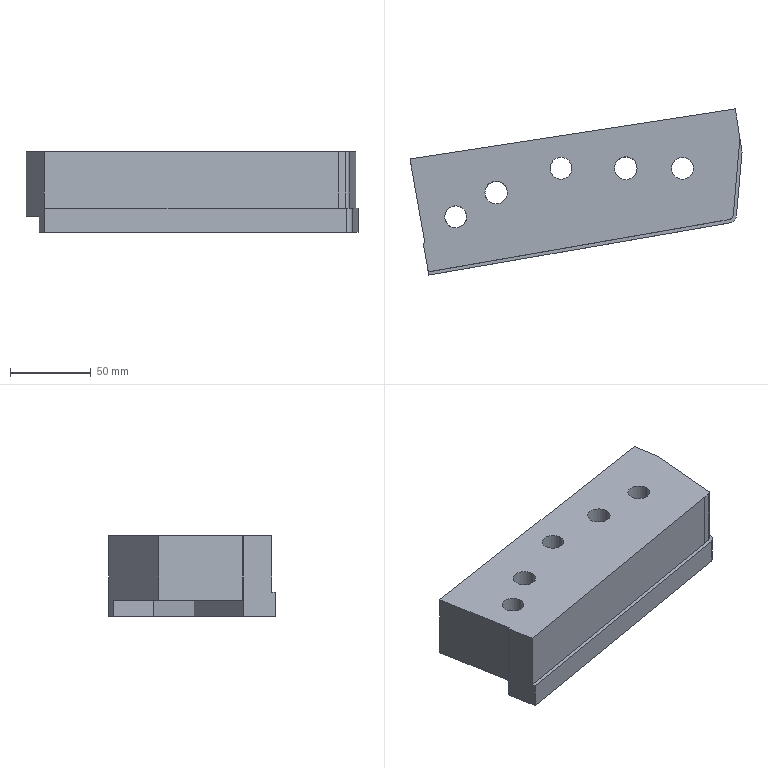Part | NX | features solid 2 | 1 solid | 29 faces | box 205.021 x 102.617 x 50 mm | volume 560361 mm3 | plane 15 | cylinder 10 | spline 4 | commonest cylinder face diameters 13.5 x3 19.5 x3 14 x2 6 x1 10 x1
STEP:
#1=CARTESIAN_POINT('',(-1109.099,373.935,43.));
#2=VERTEX_POINT('',#1);
#3=CARTESIAN_POINT('',(-1118.239,425.771,43.));
#4=VERTEX_POINT('',#3);
#5=CARTESIAN_POINT('',(-1118.069,424.808,43.));
#6=DIRECTION('',(-0.1736,0.9848,0.));
#7=VECTOR('',#6,1000.);
#8=LINE('',#5,#7);
#9=EDGE_CURVE('',#2,#4,#8,.T.);
#10=ORIENTED_EDGE('',*,*,#9,.F.);
#11=CARTESIAN_POINT('',(-1110.084,373.764,43.));
#12=VERTEX_POINT('',#11);
#13=CARTESIAN_POINT('',(-1110.084,373.764,43.));
#14=CARTESIAN_POINT('',(-1109.756,373.821,43.));
#15=CARTESIAN_POINT('',(-1109.427,373.878,43.));
#16=CARTESIAN_POINT('',(-1109.099,373.935,43.));
#17=B_SPLINE_CURVE_WITH_KNOTS('',3,(#13,#14,#15,#16),.UNSPECIFIED.,.F.,.F.,(4,4),(0.,0.001),.UNSPECIFIED.);
#18=EDGE_CURVE('',#12,#2,#17,.T.);
#19=ORIENTED_EDGE('',*,*,#18,.F.);
#20=CARTESIAN_POINT('',(-1106.958,356.037,43.));
#21=VERTEX_POINT('',#20);
#22=CARTESIAN_POINT('',(-1106.595,353.977,43.));
#23=DIRECTION('',(-0.1736,0.9848,0.));
#24=VECTOR('',#23,1000.);
#25=LINE('',#22,#24);
#26=EDGE_CURVE('',#21,#12,#25,.T.);
#27=ORIENTED_EDGE('',*,*,#26,.F.);
#28=CARTESIAN_POINT('',(-925.,387.668,43.));
#29=VERTEX_POINT('',#28);
#30=CARTESIAN_POINT('',(-1106.958,356.037,43.));
#31=CARTESIAN_POINT('',(-1103.082,356.711,43.));
#32=CARTESIAN_POINT('',(-1095.883,357.963,43.));
#33=CARTESIAN_POINT('',(-1088.27,359.287,43.));
#34=CARTESIAN_POINT('',(-1083.012,360.201,43.));
#35=CARTESIAN_POINT('',(-1079.484,360.815,43.));
#36=CARTESIAN_POINT('',(-1076.373,361.356,43.));
#37=CARTESIAN_POINT('',(-1073.677,361.825,43.));
#38=CARTESIAN_POINT('',(-1071.777,362.155,43.));
#39=CARTESIAN_POINT('',(-1070.465,362.383,43.));
#40=CARTESIAN_POINT('',(-1069.585,362.536,43.));
#41=CARTESIAN_POINT('',(-1068.808,362.671,43.));
#42=CARTESIAN_POINT('',(-1068.248,362.769,43.));
#43=CARTESIAN_POINT('',(-1067.852,362.838,43.));
#44=CARTESIAN_POINT('',(-1067.581,362.885,43.));
#45=CARTESIAN_POINT('',(-1067.377,362.92,43.));
#46=CARTESIAN_POINT('',(-1067.227,362.946,43.));
#47=CARTESIAN_POINT('',(-1067.119,362.965,43.));
#48=CARTESIAN_POINT('',(-1067.04,362.979,43.));
#49=CARTESIAN_POINT('',(-1066.968,362.991,43.));
#50=CARTESIAN_POINT('',(-1066.952,362.994,43.));
#51=CARTESIAN_POINT('',(-1066.887,363.006,43.));
#52=CARTESIAN_POINT('',(-1066.935,362.997,43.));
#53=CARTESIAN_POINT('',(-1066.64,363.048,43.));
#54=CARTESIAN_POINT('',(-1066.39,363.092,43.));
#55=CARTESIAN_POINT('',(-1065.923,363.173,43.));
#56=CARTESIAN_POINT('',(-1065.365,363.27,43.));
#57=CARTESIAN_POINT('',(-1064.01,363.506,43.));
#58=CARTESIAN_POINT('',(-1062.002,363.855,43.));
#59=CARTESIAN_POINT('',(-1059.356,364.315,43.));
#60=CARTESIAN_POINT('',(-1056.746,364.769,43.));
#61=CARTESIAN_POINT('',(-1053.314,365.366,43.));
#62=CARTESIAN_POINT('',(-1047.433,366.389,43.));
#63=CARTESIAN_POINT('',(-1039.389,367.788,43.));
#64=CARTESIAN_POINT('',(-1030.305,369.367,43.));
#65=CARTESIAN_POINT('',(-1021.793,370.848,43.));
#66=CARTESIAN_POINT('',(-1011.204,372.69,43.));
#67=CARTESIAN_POINT('',(-1001.755,374.333,43.));
#68=CARTESIAN_POINT('',(-993.448,375.778,43.));
#69=CARTESIAN_POINT('',(-987.789,376.762,43.));
#70=CARTESIAN_POINT('',(-982.699,377.648,43.));
#71=CARTESIAN_POINT('',(-978.181,378.434,43.));
#72=CARTESIAN_POINT('',(-974.891,379.006,43.));
#73=CARTESIAN_POINT('',(-972.544,379.414,43.));
#74=CARTESIAN_POINT('',(-971.196,379.649,43.));
#75=CARTESIAN_POINT('',(-970.315,379.802,43.));
#76=CARTESIAN_POINT('',(-969.83,379.887,43.));
#77=CARTESIAN_POINT('',(-969.474,379.949,43.));
#78=CARTESIAN_POINT('',(-969.13,380.008,43.));
#79=CARTESIAN_POINT('',(-968.841,380.059,43.));
#80=CARTESIAN_POINT('',(-968.662,380.09,43.));
#81=CARTESIAN_POINT('',(-968.547,380.11,43.));
#82=CARTESIAN_POINT('',(-968.525,380.114,43.));
#83=CARTESIAN_POINT('',(-968.204,380.169,43.));
#84=CARTESIAN_POINT('',(-967.907,380.221,43.));
#85=CARTESIAN_POINT('',(-967.377,380.313,43.));
#86=CARTESIAN_POINT('',(-966.482,380.469,43.));
#87=CARTESIAN_POINT('',(-965.204,380.692,43.));
#88=CARTESIAN_POINT('',(-963.2,381.04,43.));
#89=CARTESIAN_POINT('',(-960.754,381.466,43.));
#90=CARTESIAN_POINT('',(-957.921,381.959,43.));
#91=CARTESIAN_POINT('',(-954.275,382.592,43.));
#92=CARTESIAN_POINT('',(-949.967,383.341,43.));
#93=CARTESIAN_POINT('',(-945.196,384.17,43.));
#94=CARTESIAN_POINT('',(-940.823,384.93,43.));
#95=CARTESIAN_POINT('',(-935.524,385.849,43.));
#96=CARTESIAN_POINT('',(-929.895,386.825,43.));
#97=CARTESIAN_POINT('',(-926.455,387.419,43.));
#98=CARTESIAN_POINT('',(-925.,387.67,43.));
#99=B_SPLINE_CURVE_WITH_KNOTS('',3,(#30,#31,#32,#33,#34,#35,#36,#37,#38,#39,#40,#41,#42,#43,#44,#45,#46,#47,#48,#49,#50,#51,#52,#53,#54,#55,#56,#57,#58,#59,#60,#61,#62,#63,#64,#65,#66,#67,#68,#69,#70,#71,#72,#73,#74,#75,#76,#77,#78,#79,#80,#81,#82,#83,#84,#85,#86,#87,#88,#89,#90,#91,#92,#93,#94,#95,#96,#97,#98),.UNSPECIFIED.,.F.,.F.,(4,1,1,1,1,1,1,1,1,1,1,1,1,1,1,1,1,1,1,1,1,1,1,1,1,1,1,1,1,1,1,1,1,1,1,1,1,1,1,1,1,1,1,1,1,1,1,1,1,1,1,1,1,1,1,1,1,1,1,1,1,1,1,1,1,1,4),(0.2889,0.3232,0.3576,0.3747,0.3919,0.4091,0.4262,0.4434,0.452,0.4606,0.4692,0.4777,0.482,0.4863,0.4906,0.4928,0.4949,0.4971,0.4981,0.4992,0.4997,0.5,0.5003,0.5008,0.5013,0.5024,0.5035,0.5078,0.5121,0.5164,0.5207,0.5292,0.5464,0.5636,0.5808,0.5979,0.6323,0.6494,0.6666,0.6838,0.7009,0.7181,0.7267,0.7353,0.7396,0.7417,0.7439,0.746,0.7482,0.7492,0.7498,0.75,0.7503,0.7508,0.7514,0.7524,0.7546,0.7567,0.761,0.7653,0.7696,0.7782,0.7868,0.7954,0.804,0.8211,0.8383),.UNSPECIFIED.);
#100=EDGE_CURVE('',#21,#29,#99,.T.);
#101=ORIENTED_EDGE('',*,*,#100,.T.);
#102=CARTESIAN_POINT('',(-920.779,388.397,43.));
#103=VERTEX_POINT('',#102);
#104=CARTESIAN_POINT('',(-925.,387.67,43.));
#105=CARTESIAN_POINT('',(-923.175,387.985,43.));
#106=CARTESIAN_POINT('',(-921.768,388.226,43.));
#107=CARTESIAN_POINT('',(-920.779,388.395,43.));
#108=B_SPLINE_CURVE_WITH_KNOTS('',3,(#104,#105,#106,#107),.UNSPECIFIED.,.F.,.F.,(4,4),(0.8383,0.8598),.UNSPECIFIED.);
#109=EDGE_CURVE('',#29,#103,#108,.T.);
#110=ORIENTED_EDGE('',*,*,#109,.T.);
#111=CARTESIAN_POINT('',(-918.643,391.011,43.));
#112=VERTEX_POINT('',#111);
#113=CARTESIAN_POINT('',(-921.632,391.273,43.));
#114=DIRECTION('',(0.,0.,-1.));
#115=DIRECTION('',(1.,0.,0.));
#116=AXIS2_PLACEMENT_3D('',#113,#114,#115);
#117=CIRCLE('',#116,3.);
#118=EDGE_CURVE('',#112,#103,#117,.T.);
#119=ORIENTED_EDGE('',*,*,#118,.F.);
#120=CARTESIAN_POINT('',(-914.498,438.392,43.));
#121=VERTEX_POINT('',#120);
#122=CARTESIAN_POINT('',(-914.339,440.209,43.));
#123=DIRECTION('',(-0.08716,-0.9962,0.));
#124=VECTOR('',#123,1000.);
#125=LINE('',#122,#124);
#126=EDGE_CURVE('',#121,#112,#125,.T.);
#127=ORIENTED_EDGE('',*,*,#126,.F.);
#128=CARTESIAN_POINT('',(-917.312,456.685,43.));
#129=VERTEX_POINT('',#128);
#130=CARTESIAN_POINT('',(-906.384,385.652,43.));
#131=DIRECTION('',(0.1521,-0.9884,0.));
#132=VECTOR('',#131,1000.);
#133=LINE('',#130,#132);
#134=EDGE_CURVE('',#129,#121,#133,.T.);
#135=ORIENTED_EDGE('',*,*,#134,.F.);
#136=CARTESIAN_POINT('',(-1078.722,431.851,43.));
#137=DIRECTION('',(-0.9884,-0.1521,0.));
#138=VECTOR('',#137,1000.);
#139=LINE('',#136,#138);
#140=EDGE_CURVE('',#129,#4,#139,.T.);
#141=ORIENTED_EDGE('',*,*,#140,.T.);
#142=EDGE_LOOP('',(#10,#19,#27,#101,#110,#119,#127,#135,#141));
#143=FACE_BOUND('',#142,.T.);
#144=CARTESIAN_POINT('',(-1072.,405.,43.));
#145=VERTEX_POINT('',#144);
#146=CARTESIAN_POINT('',(-1065.,405.,43.));
#147=DIRECTION('',(0.,0.,-1.));
#148=DIRECTION('',(-1.,0.,0.));
#149=AXIS2_PLACEMENT_3D('',#146,#147,#148);
#150=CIRCLE('',#149,7.);
#151=EDGE_CURVE('',#145,#145,#150,.T.);
#152=ORIENTED_EDGE('',*,*,#151,.T.);
#153=EDGE_LOOP('',(#152));
#154=FACE_BOUND('',#153,.T.);
#155=CARTESIAN_POINT('',(-1096.75,390.,43.));
#156=VERTEX_POINT('',#155);
#157=CARTESIAN_POINT('',(-1090.,390.,43.));
#158=DIRECTION('',(0.,0.,-1.));
#159=DIRECTION('',(-1.,0.,0.));
#160=AXIS2_PLACEMENT_3D('',#157,#158,#159);
#161=CIRCLE('',#160,6.75);
#162=EDGE_CURVE('',#156,#156,#161,.T.);
#163=ORIENTED_EDGE('',*,*,#162,.T.);
#164=EDGE_LOOP('',(#163));
#165=FACE_BOUND('',#164,.T.);
#166=CARTESIAN_POINT('',(-1018.25,420.,43.));
#167=VERTEX_POINT('',#166);
#168=CARTESIAN_POINT('',(-1025.,420.,43.));
#169=DIRECTION('',(0.,0.,1.));
#170=DIRECTION('',(1.,0.,0.));
#171=AXIS2_PLACEMENT_3D('',#168,#169,#170);
#172=CIRCLE('',#171,6.75);
#173=EDGE_CURVE('',#167,#167,#172,.T.);
#174=ORIENTED_EDGE('',*,*,#173,.F.);
#175=EDGE_LOOP('',(#174));
#176=FACE_BOUND('',#175,.T.);
#177=CARTESIAN_POINT('',(-992.,420.,43.));
#178=VERTEX_POINT('',#177);
#179=CARTESIAN_POINT('',(-985.,420.,43.));
#180=DIRECTION('',(0.,0.,-1.));
#181=DIRECTION('',(-1.,0.,0.));
#182=AXIS2_PLACEMENT_3D('',#179,#180,#181);
#183=CIRCLE('',#182,7.);
#184=EDGE_CURVE('',#178,#178,#183,.T.);
#185=ORIENTED_EDGE('',*,*,#184,.T.);
#186=EDGE_LOOP('',(#185));
#187=FACE_BOUND('',#186,.T.);
#188=CARTESIAN_POINT('',(-956.75,420.,43.));
#189=VERTEX_POINT('',#188);
#190=CARTESIAN_POINT('',(-950.,420.,43.));
#191=DIRECTION('',(0.,0.,-1.));
#192=DIRECTION('',(-1.,0.,0.));
#193=AXIS2_PLACEMENT_3D('',#190,#191,#192);
#194=CIRCLE('',#193,6.75);
#195=EDGE_CURVE('',#189,#189,#194,.F.);
#196=ORIENTED_EDGE('',*,*,#195,.F.);
#197=EDGE_LOOP('',(#196));
#198=FACE_BOUND('',#197,.T.);
#199=CARTESIAN_POINT('',(-1067.793,360.818,43.));
#200=DIRECTION('',(0.,0.,-1.));
#201=DIRECTION('',(-1.,0.,0.));
#202=AXIS2_PLACEMENT_3D('',#199,#200,#201);
#203=PLANE('',#202);
#204=ADVANCED_FACE('',(#143,#154,#165,#176,#187,#198),#203,.F.);
#205=CARTESIAN_POINT('',(-950.,410.25,3.));
#206=VERTEX_POINT('',#205);
#207=CARTESIAN_POINT('',(-950.,420.,3.));
#208=DIRECTION('',(0.,0.,1.));
#209=DIRECTION('',(0.,-1.,0.));
#210=AXIS2_PLACEMENT_3D('',#207,#208,#209);
#211=CIRCLE('',#210,9.75);
#212=EDGE_CURVE('',#206,#206,#211,.T.);
#213=ORIENTED_EDGE('',*,*,#212,.T.);
#214=EDGE_LOOP('',(#213));
#215=FACE_BOUND('',#214,.T.);
#216=CARTESIAN_POINT('',(-1109.099,373.935,3.));
#217=VERTEX_POINT('',#216);
#218=CARTESIAN_POINT('',(-935.566,404.109,3.));
#219=VERTEX_POINT('',#218);
#220=CARTESIAN_POINT('',(-1110.084,373.764,3.));
#221=CARTESIAN_POINT('',(-1105.602,374.543,3.));
#222=CARTESIAN_POINT('',(-1101.12,375.323,3.));
#223=CARTESIAN_POINT('',(-1092.172,376.879,3.));
#224=CARTESIAN_POINT('',(-1087.705,377.656,3.));
#225=CARTESIAN_POINT('',(-1075.535,379.772,3.));
#226=CARTESIAN_POINT('',(-1067.831,381.112,3.));
#227=CARTESIAN_POINT('',(-1052.423,383.792,3.));
#228=CARTESIAN_POINT('',(-1044.719,385.131,3.));
#229=CARTESIAN_POINT('',(-1029.311,387.811,3.));
#230=CARTESIAN_POINT('',(-1021.608,389.15,3.));
#231=CARTESIAN_POINT('',(-1006.2,391.829,3.));
#232=CARTESIAN_POINT('',(-998.497,393.17,3.));
#233=CARTESIAN_POINT('',(-983.089,395.85,3.));
#234=CARTESIAN_POINT('',(-975.385,397.191,3.));
#235=CARTESIAN_POINT('',(-959.975,399.872,3.));
#236=CARTESIAN_POINT('',(-952.268,401.21,3.));
#237=CARTESIAN_POINT('',(-940.701,403.221,3.));
#238=CARTESIAN_POINT('',(-936.84,403.888,3.));
#239=CARTESIAN_POINT('',(-929.113,405.226,3.));
#240=CARTESIAN_POINT('',(-925.245,405.88,3.));
#241=CARTESIAN_POINT('',(-919.445,406.872,3.));
#242=CARTESIAN_POINT('',(-917.511,407.195,3.));
#243=CARTESIAN_POINT('',(-915.546,407.527,3.));
#244=CARTESIAN_POINT('',(-915.514,407.532,3.));
#245=CARTESIAN_POINT('',(-915.447,407.544,3.));
#246=CARTESIAN_POINT('',(-915.41,407.55,3.));
#247=CARTESIAN_POINT('',(-915.345,407.561,3.));
#248=CARTESIAN_POINT('',(-915.317,407.566,3.));
#249=CARTESIAN_POINT('',(-915.246,407.578,3.));
#250=CARTESIAN_POINT('',(-915.205,407.584,3.));
#251=CARTESIAN_POINT('',(-915.105,407.601,3.));
#252=CARTESIAN_POINT('',(-915.047,407.61,3.));
#253=CARTESIAN_POINT('',(-914.876,407.637,3.));
#254=CARTESIAN_POINT('',(-914.763,407.653,3.));
#255=CARTESIAN_POINT('',(-914.65,407.67,3.));
#256=B_SPLINE_CURVE_WITH_KNOTS('',3,(#220,#221,#222,#223,#224,#225,#226,#227,#228,#229,#230,#231,#232,#233,#234,#235,#236,#237,#238,#239,#240,#241,#242,#243,#244,#245,#246,#247,#248,#249,#250,#251,#252,#253,#254,#255),.UNSPECIFIED.,.F.,.F.,(4,2,2,2,2,2,2,2,2,2,2,2,2,2,2,2,2,4),(0.,0.05612,0.112,0.2085,0.305,0.4014,0.4979,0.5943,0.6908,0.7392,0.7875,0.8117,0.8121,0.8126,0.8129,0.8135,0.8142,0.8156),.UNSPECIFIED.);
#257=EDGE_CURVE('',#217,#219,#256,.T.);
#258=ORIENTED_EDGE('',*,*,#257,.F.);
#259=CARTESIAN_POINT('',(-1118.239,425.771,3.));
#260=VERTEX_POINT('',#259);
#261=CARTESIAN_POINT('',(-1118.069,424.808,3.));
#262=DIRECTION('',(-0.1736,0.9848,0.));
#263=VECTOR('',#262,1000.);
#264=LINE('',#261,#263);
#265=EDGE_CURVE('',#217,#260,#264,.T.);
#266=ORIENTED_EDGE('',*,*,#265,.T.);
#267=CARTESIAN_POINT('',(-937.08,453.643,3.));
#268=VERTEX_POINT('',#267);
#269=CARTESIAN_POINT('',(-896.521,459.884,3.));
#270=DIRECTION('',(-0.9884,-0.1521,0.));
#271=VECTOR('',#270,1000.);
#272=LINE('',#269,#271);
#273=EDGE_CURVE('',#268,#260,#272,.T.);
#274=ORIENTED_EDGE('',*,*,#273,.F.);
#275=CARTESIAN_POINT('',(-933.352,429.414,3.));
#276=VERTEX_POINT('',#275);
#277=CARTESIAN_POINT('',(-932.985,427.032,3.));
#278=DIRECTION('',(-0.1521,0.9884,0.));
#279=VECTOR('',#278,1000.);
#280=LINE('',#277,#279);
#281=EDGE_CURVE('',#276,#268,#280,.T.);
#282=ORIENTED_EDGE('',*,*,#281,.F.);
#283=CARTESIAN_POINT('',(-935.109,409.331,3.));
#284=DIRECTION('',(0.08716,0.9962,0.));
#285=VECTOR('',#284,1000.);
#286=LINE('',#283,#285);
#287=EDGE_CURVE('',#219,#276,#286,.T.);
#288=ORIENTED_EDGE('',*,*,#287,.F.);
#289=EDGE_LOOP('',(#258,#266,#274,#282,#288));
#290=FACE_BOUND('',#289,.T.);
#291=CARTESIAN_POINT('',(-1025.,410.25,3.));
#292=VERTEX_POINT('',#291);
#293=CARTESIAN_POINT('',(-1025.,420.,3.));
#294=DIRECTION('',(0.,0.,1.));
#295=DIRECTION('',(0.,-1.,0.));
#296=AXIS2_PLACEMENT_3D('',#293,#294,#295);
#297=CIRCLE('',#296,9.75);
#298=EDGE_CURVE('',#292,#292,#297,.F.);
#299=ORIENTED_EDGE('',*,*,#298,.F.);
#300=EDGE_LOOP('',(#299));
#301=FACE_BOUND('',#300,.T.);
#302=CARTESIAN_POINT('',(-1090.,380.25,3.));
#303=VERTEX_POINT('',#302);
#304=CARTESIAN_POINT('',(-1090.,390.,3.));
#305=DIRECTION('',(0.,0.,1.));
#306=DIRECTION('',(0.,-1.,0.));
#307=AXIS2_PLACEMENT_3D('',#304,#305,#306);
#308=CIRCLE('',#307,9.75);
#309=EDGE_CURVE('',#303,#303,#308,.T.);
#310=ORIENTED_EDGE('',*,*,#309,.T.);
#311=EDGE_LOOP('',(#310));
#312=FACE_BOUND('',#311,.T.);
#313=CARTESIAN_POINT('',(-1065.,398.,3.));
#314=VERTEX_POINT('',#313);
#315=CARTESIAN_POINT('',(-1065.,405.,3.));
#316=DIRECTION('',(0.,0.,1.));
#317=DIRECTION('',(0.,-1.,0.));
#318=AXIS2_PLACEMENT_3D('',#315,#316,#317);
#319=CIRCLE('',#318,7.);
#320=EDGE_CURVE('',#314,#314,#319,.T.);
#321=ORIENTED_EDGE('',*,*,#320,.T.);
#322=EDGE_LOOP('',(#321));
#323=FACE_BOUND('',#322,.T.);
#324=CARTESIAN_POINT('',(-992.,420.,3.));
#325=VERTEX_POINT('',#324);
#326=CARTESIAN_POINT('',(-985.,420.,3.));
#327=DIRECTION('',(0.,0.,-1.));
#328=DIRECTION('',(-1.,0.,0.));
#329=AXIS2_PLACEMENT_3D('',#326,#327,#328);
#330=CIRCLE('',#329,7.);
#331=EDGE_CURVE('',#325,#325,#330,.T.);
#332=ORIENTED_EDGE('',*,*,#331,.F.);
#333=EDGE_LOOP('',(#332));
#334=FACE_BOUND('',#333,.T.);
#335=CARTESIAN_POINT('',(-1012.373,390.756,3.));
#336=DIRECTION('',(0.,0.,1.));
#337=DIRECTION('',(0.,-1.,0.));
#338=AXIS2_PLACEMENT_3D('',#335,#336,#337);
#339=PLANE('',#338);
#340=ADVANCED_FACE('',(#215,#290,#301,#312,#323,#334),#339,.F.);
#341=CARTESIAN_POINT('',(-920.766,388.4,8.));
#342=VERTEX_POINT('',#341);
#343=CARTESIAN_POINT('',(-920.766,388.4,43.));
#344=DIRECTION('',(0.,0.,-1.));
#345=VECTOR('',#344,1000.);
#346=LINE('',#343,#345);
#347=EDGE_CURVE('',#103,#342,#346,.T.);
#348=ORIENTED_EDGE('',*,*,#347,.F.);
#349=ORIENTED_EDGE('',*,*,#109,.F.);
#350=CARTESIAN_POINT('',(-925.,387.666,8.));
#351=VERTEX_POINT('',#350);
#352=CARTESIAN_POINT('',(-925.,387.666,43.));
#353=DIRECTION('',(0.,0.,-1.));
#354=VECTOR('',#353,1000.);
#355=LINE('',#352,#354);
#356=EDGE_CURVE('',#29,#351,#355,.T.);
#357=ORIENTED_EDGE('',*,*,#356,.T.);
#358=CARTESIAN_POINT('',(-925.,387.666,8.));
#359=CARTESIAN_POINT('',(-923.589,387.914,8.));
#360=CARTESIAN_POINT('',(-922.178,388.162,8.));
#361=CARTESIAN_POINT('',(-920.766,388.4,8.));
#362=B_SPLINE_CURVE_WITH_KNOTS('',3,(#358,#359,#360,#361),.UNSPECIFIED.,.F.,.F.,(4,4),(0.,0.004294),.UNSPECIFIED.);
#363=EDGE_CURVE('',#351,#342,#362,.T.);
#364=ORIENTED_EDGE('',*,*,#363,.T.);
#365=EDGE_LOOP('',(#348,#349,#357,#364));
#366=FACE_BOUND('',#365,.T.);
#367=CARTESIAN_POINT('',(-925.,387.666,43.));
#368=CARTESIAN_POINT('',(-925.,387.666,8.));
#369=CARTESIAN_POINT('',(-923.59,387.914,43.));
#370=CARTESIAN_POINT('',(-923.59,387.914,8.));
#371=CARTESIAN_POINT('',(-922.18,388.162,43.));
#372=CARTESIAN_POINT('',(-922.18,388.162,8.));
#373=CARTESIAN_POINT('',(-920.766,388.4,43.));
#374=CARTESIAN_POINT('',(-920.766,388.4,8.));
#375=B_SPLINE_SURFACE_WITH_KNOTS('',3,1,((#367,#368),(#369,#370),(#371,#372),(#373,#374)),.SURF_OF_LINEAR_EXTRUSION.,.F.,.F.,.F.,(4,4),(2,2),(0.8587,0.8694),(0.,1.),.PIECEWISE_BEZIER_KNOTS.);
#376=ADVANCED_FACE('',(#366),#375,.F.);
#377=ORIENTED_EDGE('',*,*,#273,.T.);
#378=CARTESIAN_POINT('',(-1118.239,425.771,43.));
#379=DIRECTION('',(0.,0.,1.));
#380=VECTOR('',#379,1000.);
#381=LINE('',#378,#380);
#382=EDGE_CURVE('',#260,#4,#381,.T.);
#383=ORIENTED_EDGE('',*,*,#382,.T.);
#384=ORIENTED_EDGE('',*,*,#140,.F.);
#385=CARTESIAN_POINT('',(-917.312,456.685,-7.));
#386=VERTEX_POINT('',#385);
#387=CARTESIAN_POINT('',(-917.312,456.685,43.));
#388=DIRECTION('',(0.,0.,1.));
#389=VECTOR('',#388,1000.);
#390=LINE('',#387,#389);
#391=EDGE_CURVE('',#386,#129,#390,.T.);
#392=ORIENTED_EDGE('',*,*,#391,.F.);
#393=CARTESIAN_POINT('',(-937.08,453.643,-7.));
#394=VERTEX_POINT('',#393);
#395=CARTESIAN_POINT('',(-1078.722,431.851,-7.));
#396=DIRECTION('',(-0.9884,-0.1521,0.));
#397=VECTOR('',#396,1000.);
#398=LINE('',#395,#397);
#399=EDGE_CURVE('',#386,#394,#398,.T.);
#400=ORIENTED_EDGE('',*,*,#399,.T.);
#401=CARTESIAN_POINT('',(-937.08,453.643,43.));
#402=DIRECTION('',(0.,0.,-1.));
#403=VECTOR('',#402,1000.);
#404=LINE('',#401,#403);
#405=EDGE_CURVE('',#268,#394,#404,.T.);
#406=ORIENTED_EDGE('',*,*,#405,.F.);
#407=EDGE_LOOP('',(#377,#383,#384,#392,#400,#406));
#408=FACE_BOUND('',#407,.T.);
#409=CARTESIAN_POINT('',(-896.521,459.884,43.));
#410=DIRECTION('',(0.1521,-0.9884,0.));
#411=DIRECTION('',(0.9884,0.1521,0.));
#412=AXIS2_PLACEMENT_3D('',#409,#410,#411);
#413=PLANE('',#412);
#414=ADVANCED_FACE('',(#408),#413,.F.);
#415=CARTESIAN_POINT('',(-1110.084,373.764,-7.));
#416=VERTEX_POINT('',#415);
#417=CARTESIAN_POINT('',(-935.566,404.109,-7.));
#418=VERTEX_POINT('',#417);
#419=CARTESIAN_POINT('',(-1110.084,373.764,-7.));
#420=CARTESIAN_POINT('',(-1105.602,374.543,-7.));
#421=CARTESIAN_POINT('',(-1101.12,375.323,-7.));
#422=CARTESIAN_POINT('',(-1092.172,376.879,-7.));
#423=CARTESIAN_POINT('',(-1087.705,377.656,-7.));
#424=CARTESIAN_POINT('',(-1075.535,379.772,-7.));
#425=CARTESIAN_POINT('',(-1067.831,381.112,-7.));
#426=CARTESIAN_POINT('',(-1052.423,383.792,-7.));
#427=CARTESIAN_POINT('',(-1044.719,385.131,-7.));
#428=CARTESIAN_POINT('',(-1029.311,387.811,-7.));
#429=CARTESIAN_POINT('',(-1021.608,389.15,-7.));
#430=CARTESIAN_POINT('',(-1006.2,391.829,-7.));
#431=CARTESIAN_POINT('',(-998.497,393.17,-7.));
#432=CARTESIAN_POINT('',(-983.089,395.85,-7.));
#433=CARTESIAN_POINT('',(-975.385,397.191,-7.));
#434=CARTESIAN_POINT('',(-959.975,399.872,-7.));
#435=CARTESIAN_POINT('',(-952.268,401.21,-7.));
#436=CARTESIAN_POINT('',(-940.701,403.221,-7.));
#437=CARTESIAN_POINT('',(-936.84,403.888,-7.));
#438=CARTESIAN_POINT('',(-929.113,405.226,-7.));
#439=CARTESIAN_POINT('',(-925.245,405.88,-7.));
#440=CARTESIAN_POINT('',(-919.445,406.872,-7.));
#441=CARTESIAN_POINT('',(-917.511,407.195,-7.));
#442=CARTESIAN_POINT('',(-915.546,407.527,-7.));
#443=CARTESIAN_POINT('',(-915.514,407.532,-7.));
#444=CARTESIAN_POINT('',(-915.447,407.544,-7.));
#445=CARTESIAN_POINT('',(-915.41,407.55,-7.));
#446=CARTESIAN_POINT('',(-915.345,407.561,-7.));
#447=CARTESIAN_POINT('',(-915.317,407.566,-7.));
#448=CARTESIAN_POINT('',(-915.246,407.578,-7.));
#449=CARTESIAN_POINT('',(-915.205,407.584,-7.));
#450=CARTESIAN_POINT('',(-915.105,407.601,-7.));
#451=CARTESIAN_POINT('',(-915.047,407.61,-7.));
#452=CARTESIAN_POINT('',(-914.876,407.637,-7.));
#453=CARTESIAN_POINT('',(-914.763,407.653,-7.));
#454=CARTESIAN_POINT('',(-914.65,407.67,-7.));
#455=B_SPLINE_CURVE_WITH_KNOTS('',3,(#419,#420,#421,#422,#423,#424,#425,#426,#427,#428,#429,#430,#431,#432,#433,#434,#435,#436,#437,#438,#439,#440,#441,#442,#443,#444,#445,#446,#447,#448,#449,#450,#451,#452,#453,#454),.UNSPECIFIED.,.F.,.F.,(4,2,2,2,2,2,2,2,2,2,2,2,2,2,2,2,2,4),(0.,0.05612,0.112,0.2085,0.305,0.4014,0.4979,0.5943,0.6908,0.7392,0.7875,0.8117,0.8121,0.8126,0.8129,0.8135,0.8142,0.8156),.UNSPECIFIED.);
#456=EDGE_CURVE('',#416,#418,#455,.T.);
#457=ORIENTED_EDGE('',*,*,#456,.T.);
#458=CARTESIAN_POINT('',(-933.352,429.414,-7.));
#459=VERTEX_POINT('',#458);
#460=CARTESIAN_POINT('',(-935.109,409.331,-7.));
#461=DIRECTION('',(0.08716,0.9962,0.));
#462=VECTOR('',#461,1000.);
#463=LINE('',#460,#462);
#464=EDGE_CURVE('',#418,#459,#463,.T.);
#465=ORIENTED_EDGE('',*,*,#464,.T.);
#466=CARTESIAN_POINT('',(-932.985,427.032,-7.));
#467=DIRECTION('',(-0.1521,0.9884,0.));
#468=VECTOR('',#467,1000.);
#469=LINE('',#466,#468);
#470=EDGE_CURVE('',#459,#394,#469,.T.);
#471=ORIENTED_EDGE('',*,*,#470,.T.);
#472=ORIENTED_EDGE('',*,*,#399,.F.);
#473=CARTESIAN_POINT('',(-913.218,430.073,-7.));
#474=VERTEX_POINT('',#473);
#475=CARTESIAN_POINT('',(-909.884,408.403,-7.));
#476=DIRECTION('',(-0.1521,0.9884,0.));
#477=VECTOR('',#476,1000.);
#478=LINE('',#475,#477);
#479=EDGE_CURVE('',#474,#386,#478,.T.);
#480=ORIENTED_EDGE('',*,*,#479,.F.);
#481=CARTESIAN_POINT('',(-916.651,390.837,-7.));
#482=VERTEX_POINT('',#481);
#483=CARTESIAN_POINT('',(-920.405,347.924,-7.));
#484=DIRECTION('',(-0.08716,-0.9962,0.));
#485=VECTOR('',#484,1000.);
#486=LINE('',#483,#485);
#487=EDGE_CURVE('',#474,#482,#486,.T.);
#488=ORIENTED_EDGE('',*,*,#487,.T.);
#489=CARTESIAN_POINT('',(-920.475,386.408,-7.));
#490=VERTEX_POINT('',#489);
#491=CARTESIAN_POINT('',(-921.632,391.273,-7.));
#492=DIRECTION('',(0.,0.,-1.));
#493=DIRECTION('',(-1.,0.,0.));
#494=AXIS2_PLACEMENT_3D('',#491,#492,#493);
#495=CIRCLE('',#494,5.);
#496=EDGE_CURVE('',#482,#490,#495,.T.);
#497=ORIENTED_EDGE('',*,*,#496,.T.);
#498=CARTESIAN_POINT('',(-1106.611,354.067,-7.));
#499=VERTEX_POINT('',#498);
#500=CARTESIAN_POINT('',(-1263.358,326.807,-7.));
#501=CARTESIAN_POINT('',(-1232.991,332.088,-7.));
#502=CARTESIAN_POINT('',(-1171.809,342.729,-7.));
#503=CARTESIAN_POINT('',(-1095.22,356.049,-7.));
#504=CARTESIAN_POINT('',(-1033.589,366.767,-7.));
#505=CARTESIAN_POINT('',(-987.365,374.804,-7.));
#506=CARTESIAN_POINT('',(-948.847,381.509,-7.));
#507=CARTESIAN_POINT('',(-923.808,385.853,-7.));
#508=CARTESIAN_POINT('',(-914.109,387.486,-7.));
#509=CARTESIAN_POINT('',(-912.091,387.827,-7.));
#510=CARTESIAN_POINT('',(-911.971,387.848,-7.));
#511=CARTESIAN_POINT('',(-911.79,387.876,-7.));
#512=CARTESIAN_POINT('',(-911.394,387.917,-7.));
#513=CARTESIAN_POINT('',(-910.546,388.022,-7.));
#514=CARTESIAN_POINT('',(-908.847,388.221,-7.));
#515=CARTESIAN_POINT('',(-906.42,388.511,-7.));
#516=CARTESIAN_POINT('',(-903.994,388.799,-7.));
#517=CARTESIAN_POINT('',(-902.295,389.001,-7.));
#518=CARTESIAN_POINT('',(-901.446,389.101,-7.));
#519=CARTESIAN_POINT('',(-901.052,389.148,-7.));
#520=CARTESIAN_POINT('',(-900.87,389.17,-7.));
#521=CARTESIAN_POINT('',(-900.748,389.184,-7.));
#522=CARTESIAN_POINT('',(-899.68,389.239,-7.));
#523=CARTESIAN_POINT('',(-897.973,389.35,-7.));
#524=CARTESIAN_POINT('',(-896.023,389.486,-7.));
#525=CARTESIAN_POINT('',(-894.456,389.561,-7.));
#526=CARTESIAN_POINT('',(-892.989,389.903,-7.));
#527=CARTESIAN_POINT('',(-891.495,390.907,-7.));
#528=CARTESIAN_POINT('',(-890.458,392.378,-7.));
#529=CARTESIAN_POINT('',(-890.077,393.863,-7.));
#530=CARTESIAN_POINT('',(-889.825,397.101,-7.));
#531=CARTESIAN_POINT('',(-889.362,402.393,-7.));
#532=CARTESIAN_POINT('',(-888.928,407.354,-7.));
#533=CARTESIAN_POINT('',(-888.696,410.,-7.));
#534=B_SPLINE_CURVE_WITH_KNOTS('',3,(#500,#501,#502,#503,#504,#505,#506,#507,#508,#509,#510,#511,#512,#513,#514,#515,#516,#517,#518,#519,#520,#521,#522,#523,#524,#525,#526,#527,#528,#529,#530,#531,#532,#533),.UNSPECIFIED.,.F.,.F.,(4,1,1,1,1,1,1,1,1,1,1,1,1,1,1,1,1,1,1,1,1,1,1,1,1,1,1,1,1,1,1,4),(0.,0.2329,0.4693,0.5875,0.7056,0.8238,0.8829,0.8977,0.8981,0.8984,0.8986,0.8995,0.9014,0.9051,0.9124,0.9198,0.9235,0.9254,0.9263,0.9265,0.9268,0.9272,0.9346,0.9397,0.942,0.9465,0.9509,0.9554,0.9599,0.9624,0.9799,1.),.UNSPECIFIED.);
#535=EDGE_CURVE('',#499,#490,#534,.T.);
#536=ORIENTED_EDGE('',*,*,#535,.F.);
#537=CARTESIAN_POINT('',(-1106.595,353.977,-7.));
#538=DIRECTION('',(-0.1736,0.9848,0.));
#539=VECTOR('',#538,1000.);
#540=LINE('',#537,#539);
#541=EDGE_CURVE('',#499,#416,#540,.T.);
#542=ORIENTED_EDGE('',*,*,#541,.T.);
#543=EDGE_LOOP('',(#457,#465,#471,#472,#480,#488,#497,#536,#542));
#544=FACE_BOUND('',#543,.T.);
#545=CARTESIAN_POINT('',(-1067.793,360.818,-7.));
#546=DIRECTION('',(0.,0.,-1.));
#547=DIRECTION('',(-1.,0.,0.));
#548=AXIS2_PLACEMENT_3D('',#545,#546,#547);
#549=PLANE('',#548);
#550=ADVANCED_FACE('',(#544),#549,.T.);
#551=CARTESIAN_POINT('',(-1106.611,354.067,8.));
#552=VERTEX_POINT('',#551);
#553=CARTESIAN_POINT('',(-920.475,386.408,8.));
#554=VERTEX_POINT('',#553);
#555=CARTESIAN_POINT('',(-1106.611,354.067,8.));
#556=CARTESIAN_POINT('',(-1075.589,359.463,8.));
#557=CARTESIAN_POINT('',(-1029.057,367.559,8.));
#558=CARTESIAN_POINT('',(-967.011,378.336,8.));
#559=CARTESIAN_POINT('',(-935.995,383.767,8.));
#560=CARTESIAN_POINT('',(-920.475,386.408,8.));
#561=B_SPLINE_CURVE_WITH_KNOTS('',3,(#555,#556,#557,#558,#559,#560),.UNSPECIFIED.,.F.,.F.,(4,1,1,4),(1.747,1.842,1.889,1.936),.UNSPECIFIED.);
#562=EDGE_CURVE('',#552,#554,#561,.T.);
#563=ORIENTED_EDGE('',*,*,#562,.T.);
#564=CARTESIAN_POINT('',(-916.651,390.837,8.));
#565=VERTEX_POINT('',#564);
#566=CARTESIAN_POINT('',(-921.632,391.273,8.));
#567=DIRECTION('',(0.,0.,1.));
#568=DIRECTION('',(1.,0.,0.));
#569=AXIS2_PLACEMENT_3D('',#566,#567,#568);
#570=CIRCLE('',#569,5.);
#571=EDGE_CURVE('',#554,#565,#570,.T.);
#572=ORIENTED_EDGE('',*,*,#571,.T.);
#573=CARTESIAN_POINT('',(-913.218,430.073,8.));
#574=VERTEX_POINT('',#573);
#575=CARTESIAN_POINT('',(-916.651,390.837,8.));
#576=DIRECTION('',(-0.08716,-0.9962,0.));
#577=VECTOR('',#576,1000.);
#578=LINE('',#575,#577);
#579=EDGE_CURVE('',#565,#574,#578,.F.);
#580=ORIENTED_EDGE('',*,*,#579,.T.);
#581=CARTESIAN_POINT('',(-914.498,438.392,8.));
#582=VERTEX_POINT('',#581);
#583=CARTESIAN_POINT('',(-913.218,430.073,8.));
#584=DIRECTION('',(0.1521,-0.9884,0.));
#585=VECTOR('',#584,1000.);
#586=LINE('',#583,#585);
#587=EDGE_CURVE('',#574,#582,#586,.F.);
#588=ORIENTED_EDGE('',*,*,#587,.T.);
#589=CARTESIAN_POINT('',(-918.643,391.011,8.));
#590=VERTEX_POINT('',#589);
#591=CARTESIAN_POINT('',(-925.728,310.033,8.));
#592=DIRECTION('',(0.08716,0.9962,0.));
#593=VECTOR('',#592,1000.);
#594=LINE('',#591,#593);
#595=EDGE_CURVE('',#582,#590,#594,.F.);
#596=ORIENTED_EDGE('',*,*,#595,.T.);
#597=CARTESIAN_POINT('',(-921.632,391.273,8.));
#598=DIRECTION('',(0.,0.,-1.));
#599=DIRECTION('',(1.,0.,0.));
#600=AXIS2_PLACEMENT_3D('',#597,#598,#599);
#601=CIRCLE('',#600,3.);
#602=EDGE_CURVE('',#590,#342,#601,.T.);
#603=ORIENTED_EDGE('',*,*,#602,.T.);
#604=ORIENTED_EDGE('',*,*,#363,.F.);
#605=CARTESIAN_POINT('',(-1106.959,356.038,8.));
#606=VERTEX_POINT('',#605);
#607=CARTESIAN_POINT('',(-1106.959,356.038,8.));
#608=CARTESIAN_POINT('',(-1076.633,361.312,8.));
#609=CARTESIAN_POINT('',(-1015.975,371.826,8.));
#610=CARTESIAN_POINT('',(-955.337,382.457,8.));
#611=CARTESIAN_POINT('',(-925.,387.666,8.));
#612=B_SPLINE_CURVE_WITH_KNOTS('',3,(#607,#608,#609,#610,#611),.UNSPECIFIED.,.F.,.F.,(4,1,4),(1.695,1.787,1.879),.UNSPECIFIED.);
#613=EDGE_CURVE('',#606,#351,#612,.T.);
#614=ORIENTED_EDGE('',*,*,#613,.F.);
#615=CARTESIAN_POINT('',(-1108.407,364.255,8.));
#616=DIRECTION('',(0.1736,-0.9848,0.));
#617=VECTOR('',#616,1000.);
#618=LINE('',#615,#617);
#619=EDGE_CURVE('',#606,#552,#618,.T.);
#620=ORIENTED_EDGE('',*,*,#619,.T.);
#621=EDGE_LOOP('',(#563,#572,#580,#588,#596,#603,#604,#614,#620));
#622=FACE_BOUND('',#621,.T.);
#623=CARTESIAN_POINT('',(-1253.358,338.697,8.));
#624=DIRECTION('',(0.,0.,1.));
#625=DIRECTION('',(1.,0.,0.));
#626=AXIS2_PLACEMENT_3D('',#623,#624,#625);
#627=PLANE('',#626);
#628=ADVANCED_FACE('',(#622),#627,.T.);
#629=CARTESIAN_POINT('',(-920.475,386.408,0.5));
#630=DIRECTION('',(0.,0.,-1.));
#631=VECTOR('',#630,1000.);
#632=LINE('',#629,#631);
#633=EDGE_CURVE('',#554,#490,#632,.T.);
#634=ORIENTED_EDGE('',*,*,#633,.F.);
#635=ORIENTED_EDGE('',*,*,#562,.F.);
#636=CARTESIAN_POINT('',(-1106.611,354.067,0.5));
#637=DIRECTION('',(0.,0.,-1.));
#638=VECTOR('',#637,1000.);
#639=LINE('',#636,#638);
#640=EDGE_CURVE('',#499,#552,#639,.F.);
#641=ORIENTED_EDGE('',*,*,#640,.F.);
#642=ORIENTED_EDGE('',*,*,#535,.T.);
#643=EDGE_LOOP('',(#634,#635,#641,#642));
#644=FACE_BOUND('',#643,.T.);
#645=CARTESIAN_POINT('',(-1106.611,354.067,8.));
#646=CARTESIAN_POINT('',(-1106.611,354.067,-7.));
#647=CARTESIAN_POINT('',(-1075.589,359.463,8.));
#648=CARTESIAN_POINT('',(-1075.589,359.463,-7.));
#649=CARTESIAN_POINT('',(-1029.057,367.559,8.));
#650=CARTESIAN_POINT('',(-1029.057,367.559,-7.));
#651=CARTESIAN_POINT('',(-967.011,378.336,8.));
#652=CARTESIAN_POINT('',(-967.011,378.336,-7.));
#653=CARTESIAN_POINT('',(-935.995,383.767,8.));
#654=CARTESIAN_POINT('',(-935.995,383.767,-7.));
#655=CARTESIAN_POINT('',(-920.475,386.408,8.));
#656=CARTESIAN_POINT('',(-920.475,386.408,-7.));
#657=B_SPLINE_SURFACE_WITH_KNOTS('',3,1,((#645,#646),(#647,#648),(#649,#650),(#651,#652),(#653,#654),(#655,#656)),.SURF_OF_LINEAR_EXTRUSION.,.F.,.F.,.F.,(4,1,1,4),(2,2),(0.4008,0.6387,0.7577,0.8766),(0.,1.),.UNSPECIFIED.);
#658=ADVANCED_FACE('',(#644),#657,.F.);
#659=CARTESIAN_POINT('',(-935.566,404.109,-2.));
#660=DIRECTION('',(0.,0.,-1.));
#661=VECTOR('',#660,1000.);
#662=LINE('',#659,#661);
#663=EDGE_CURVE('',#219,#418,#662,.T.);
#664=ORIENTED_EDGE('',*,*,#663,.T.);
#665=ORIENTED_EDGE('',*,*,#456,.F.);
#666=CARTESIAN_POINT('',(-1110.084,373.764,3.));
#667=DIRECTION('',(0.,0.,-1.));
#668=VECTOR('',#667,1000.);
#669=LINE('',#666,#668);
#670=EDGE_CURVE('',#12,#416,#669,.T.);
#671=ORIENTED_EDGE('',*,*,#670,.F.);
#672=ORIENTED_EDGE('',*,*,#18,.T.);
#673=CARTESIAN_POINT('',(-1109.099,373.935,23.));
#674=DIRECTION('',(0.,0.,-1.));
#675=VECTOR('',#674,1000.);
#676=LINE('',#673,#675);
#677=EDGE_CURVE('',#2,#217,#676,.T.);
#678=ORIENTED_EDGE('',*,*,#677,.T.);
#679=ORIENTED_EDGE('',*,*,#257,.T.);
#680=EDGE_LOOP('',(#664,#665,#671,#672,#678,#679));
#681=FACE_BOUND('',#680,.T.);
#682=CARTESIAN_POINT('',(-1110.084,373.764,43.));
#683=CARTESIAN_POINT('',(-1110.084,373.764,-7.));
#684=CARTESIAN_POINT('',(-1051.912,383.881,43.));
#685=CARTESIAN_POINT('',(-1051.912,383.881,-7.));
#686=CARTESIAN_POINT('',(-993.747,394.04,43.));
#687=CARTESIAN_POINT('',(-993.747,394.04,-7.));
#688=CARTESIAN_POINT('',(-935.566,404.109,43.));
#689=CARTESIAN_POINT('',(-935.566,404.109,-7.));
#690=B_SPLINE_SURFACE_WITH_KNOTS('',3,1,((#682,#683),(#684,#685),(#686,#687),(#688,#689)),.SURF_OF_LINEAR_EXTRUSION.,.F.,.F.,.F.,(4,4),(2,2),(0.,0.7284),(0.,1.),.PIECEWISE_BEZIER_KNOTS.);
#691=ADVANCED_FACE('',(#681),#690,.T.);
#692=ORIENTED_EDGE('',*,*,#26,.T.);
#693=ORIENTED_EDGE('',*,*,#670,.T.);
#694=ORIENTED_EDGE('',*,*,#541,.F.);
#695=ORIENTED_EDGE('',*,*,#640,.T.);
#696=ORIENTED_EDGE('',*,*,#619,.F.);
#697=CARTESIAN_POINT('',(-1106.959,356.038,43.));
#698=DIRECTION('',(0.,0.,-1.));
#699=VECTOR('',#698,1000.);
#700=LINE('',#697,#699);
#701=EDGE_CURVE('',#606,#21,#700,.F.);
#702=ORIENTED_EDGE('',*,*,#701,.T.);
#703=EDGE_LOOP('',(#692,#693,#694,#695,#696,#702));
#704=FACE_BOUND('',#703,.T.);
#705=CARTESIAN_POINT('',(-1120.,430.,-57.));
#706=DIRECTION('',(-0.9848,-0.1736,0.));
#707=DIRECTION('',(0.1736,-0.9848,0.));
#708=AXIS2_PLACEMENT_3D('',#705,#706,#707);
#709=PLANE('',#708);
#710=ADVANCED_FACE('',(#704),#709,.T.);
#711=CARTESIAN_POINT('',(-1018.25,420.,18.));
#712=VERTEX_POINT('',#711);
#713=CARTESIAN_POINT('',(-1025.,420.,18.));
#714=DIRECTION('',(0.,0.,1.));
#715=DIRECTION('',(1.,0.,0.));
#716=AXIS2_PLACEMENT_3D('',#713,#714,#715);
#717=CIRCLE('',#716,6.75);
#718=EDGE_CURVE('',#712,#712,#717,.T.);
#719=ORIENTED_EDGE('',*,*,#718,.T.);
#720=EDGE_LOOP('',(#719));
#721=FACE_BOUND('',#720,.T.);
#722=CARTESIAN_POINT('',(-1015.25,420.,18.));
#723=VERTEX_POINT('',#722);
#724=CARTESIAN_POINT('',(-1025.,420.,18.));
#725=DIRECTION('',(0.,0.,1.));
#726=DIRECTION('',(1.,0.,0.));
#727=AXIS2_PLACEMENT_3D('',#724,#725,#726);
#728=CIRCLE('',#727,9.75);
#729=EDGE_CURVE('',#723,#723,#728,.T.);
#730=ORIENTED_EDGE('',*,*,#729,.F.);
#731=EDGE_LOOP('',(#730));
#732=FACE_BOUND('',#731,.T.);
#733=CARTESIAN_POINT('',(-1025.,420.,18.));
#734=DIRECTION('',(0.,0.,1.));
#735=DIRECTION('',(1.,0.,0.));
#736=AXIS2_PLACEMENT_3D('',#733,#734,#735);
#737=PLANE('',#736);
#738=ADVANCED_FACE('',(#721,#732),#737,.F.);
#739=ORIENTED_EDGE('',*,*,#173,.T.);
#740=EDGE_LOOP('',(#739));
#741=FACE_BOUND('',#740,.T.);
#742=ORIENTED_EDGE('',*,*,#718,.F.);
#743=EDGE_LOOP('',(#742));
#744=FACE_BOUND('',#743,.T.);
#745=CARTESIAN_POINT('',(-1025.,420.,43.));
#746=DIRECTION('',(0.,0.,1.));
#747=DIRECTION('',(1.,0.,0.));
#748=AXIS2_PLACEMENT_3D('',#745,#746,#747);
#749=CYLINDRICAL_SURFACE('',#748,6.75);
#750=ADVANCED_FACE('',(#741,#744),#749,.F.);
#751=ORIENTED_EDGE('',*,*,#298,.T.);
#752=EDGE_LOOP('',(#751));
#753=FACE_BOUND('',#752,.T.);
#754=ORIENTED_EDGE('',*,*,#729,.T.);
#755=EDGE_LOOP('',(#754));
#756=FACE_BOUND('',#755,.T.);
#757=CARTESIAN_POINT('',(-1025.,420.,-7.));
#758=DIRECTION('',(0.,0.,1.));
#759=DIRECTION('',(1.,0.,0.));
#760=AXIS2_PLACEMENT_3D('',#757,#758,#759);
#761=CYLINDRICAL_SURFACE('',#760,9.75);
#762=ADVANCED_FACE('',(#753,#756),#761,.F.);
#763=ORIENTED_EDGE('',*,*,#701,.F.);
#764=ORIENTED_EDGE('',*,*,#613,.T.);
#765=ORIENTED_EDGE('',*,*,#356,.F.);
#766=ORIENTED_EDGE('',*,*,#100,.F.);
#767=EDGE_LOOP('',(#763,#764,#765,#766));
#768=FACE_BOUND('',#767,.T.);
#769=CARTESIAN_POINT('',(-1106.959,356.038,43.));
#770=CARTESIAN_POINT('',(-1106.959,356.038,8.));
#771=CARTESIAN_POINT('',(-1076.633,361.312,43.));
#772=CARTESIAN_POINT('',(-1076.633,361.312,8.));
#773=CARTESIAN_POINT('',(-1015.975,371.826,43.));
#774=CARTESIAN_POINT('',(-1015.975,371.826,8.));
#775=CARTESIAN_POINT('',(-955.337,382.457,43.));
#776=CARTESIAN_POINT('',(-955.337,382.457,8.));
#777=CARTESIAN_POINT('',(-925.,387.666,43.));
#778=CARTESIAN_POINT('',(-925.,387.666,8.));
#779=B_SPLINE_SURFACE_WITH_KNOTS('',3,1,((#769,#770),(#771,#772),(#773,#774),(#775,#776),(#777,#778)),.SURF_OF_LINEAR_EXTRUSION.,.F.,.F.,.F.,(4,1,4),(2,2),(0.3805,0.6192,0.8579),(0.,1.),.UNSPECIFIED.);
#780=ADVANCED_FACE('',(#768),#779,.F.);
#781=CARTESIAN_POINT('',(-1090.,383.25,18.));
#782=VERTEX_POINT('',#781);
#783=CARTESIAN_POINT('',(-1090.,390.,18.));
#784=DIRECTION('',(0.,0.,1.));
#785=DIRECTION('',(0.,-1.,0.));
#786=AXIS2_PLACEMENT_3D('',#783,#784,#785);
#787=CIRCLE('',#786,6.75);
#788=EDGE_CURVE('',#782,#782,#787,.T.);
#789=ORIENTED_EDGE('',*,*,#788,.F.);
#790=EDGE_LOOP('',(#789));
#791=FACE_BOUND('',#790,.T.);
#792=ORIENTED_EDGE('',*,*,#162,.F.);
#793=EDGE_LOOP('',(#792));
#794=FACE_BOUND('',#793,.T.);
#795=CARTESIAN_POINT('',(-1090.,390.,53.));
#796=DIRECTION('',(0.,0.,1.));
#797=DIRECTION('',(0.,-1.,0.));
#798=AXIS2_PLACEMENT_3D('',#795,#796,#797);
#799=CYLINDRICAL_SURFACE('',#798,6.75);
#800=ADVANCED_FACE('',(#791,#794),#799,.F.);
#801=ORIENTED_EDGE('',*,*,#788,.T.);
#802=EDGE_LOOP('',(#801));
#803=FACE_BOUND('',#802,.T.);
#804=CARTESIAN_POINT('',(-1090.,380.25,18.));
#805=VERTEX_POINT('',#804);
#806=CARTESIAN_POINT('',(-1090.,390.,18.));
#807=DIRECTION('',(0.,0.,1.));
#808=DIRECTION('',(0.,-1.,0.));
#809=AXIS2_PLACEMENT_3D('',#806,#807,#808);
#810=CIRCLE('',#809,9.75);
#811=EDGE_CURVE('',#805,#805,#810,.T.);
#812=ORIENTED_EDGE('',*,*,#811,.F.);
#813=EDGE_LOOP('',(#812));
#814=FACE_BOUND('',#813,.T.);
#815=CARTESIAN_POINT('',(-1090.,390.,18.));
#816=DIRECTION('',(0.,0.,1.));
#817=DIRECTION('',(0.,-1.,0.));
#818=AXIS2_PLACEMENT_3D('',#815,#816,#817);
#819=PLANE('',#818);
#820=ADVANCED_FACE('',(#803,#814),#819,.F.);
#821=ORIENTED_EDGE('',*,*,#811,.T.);
#822=EDGE_LOOP('',(#821));
#823=FACE_BOUND('',#822,.T.);
#824=ORIENTED_EDGE('',*,*,#309,.F.);
#825=EDGE_LOOP('',(#824));
#826=FACE_BOUND('',#825,.T.);
#827=CARTESIAN_POINT('',(-1090.,390.,3.));
#828=DIRECTION('',(0.,0.,1.));
#829=DIRECTION('',(0.,-1.,0.));
#830=AXIS2_PLACEMENT_3D('',#827,#828,#829);
#831=CYLINDRICAL_SURFACE('',#830,9.75);
#832=ADVANCED_FACE('',(#823,#826),#831,.F.);
#833=ORIENTED_EDGE('',*,*,#320,.F.);
#834=EDGE_LOOP('',(#833));
#835=FACE_BOUND('',#834,.T.);
#836=ORIENTED_EDGE('',*,*,#151,.F.);
#837=EDGE_LOOP('',(#836));
#838=FACE_BOUND('',#837,.T.);
#839=CARTESIAN_POINT('',(-1065.,405.,3.));
#840=DIRECTION('',(0.,0.,1.));
#841=DIRECTION('',(0.,-1.,0.));
#842=AXIS2_PLACEMENT_3D('',#839,#840,#841);
#843=CYLINDRICAL_SURFACE('',#842,7.);
#844=ADVANCED_FACE('',(#835,#838),#843,.F.);
#845=ORIENTED_EDGE('',*,*,#487,.F.);
#846=CARTESIAN_POINT('',(-913.218,430.073,-457.));
#847=DIRECTION('',(0.,0.,1.));
#848=VECTOR('',#847,1000.);
#849=LINE('',#846,#848);
#850=EDGE_CURVE('',#474,#574,#849,.T.);
#851=ORIENTED_EDGE('',*,*,#850,.T.);
#852=ORIENTED_EDGE('',*,*,#579,.F.);
#853=CARTESIAN_POINT('',(-916.651,390.837,-50.));
#854=DIRECTION('',(0.,0.,1.));
#855=VECTOR('',#854,1000.);
#856=LINE('',#853,#855);
#857=EDGE_CURVE('',#482,#565,#856,.T.);
#858=ORIENTED_EDGE('',*,*,#857,.F.);
#859=EDGE_LOOP('',(#845,#851,#852,#858));
#860=FACE_BOUND('',#859,.T.);
#861=CARTESIAN_POINT('',(-916.651,390.837,-50.));
#862=DIRECTION('',(0.9962,-0.08716,0.));
#863=DIRECTION('',(0.08716,0.9962,0.));
#864=AXIS2_PLACEMENT_3D('',#861,#862,#863);
#865=PLANE('',#864);
#866=ADVANCED_FACE('',(#860),#865,.T.);
#867=ORIENTED_EDGE('',*,*,#857,.T.);
#868=ORIENTED_EDGE('',*,*,#571,.F.);
#869=ORIENTED_EDGE('',*,*,#633,.T.);
#870=ORIENTED_EDGE('',*,*,#496,.F.);
#871=EDGE_LOOP('',(#867,#868,#869,#870));
#872=FACE_BOUND('',#871,.T.);
#873=CARTESIAN_POINT('',(-921.632,391.273,-50.));
#874=DIRECTION('',(0.,0.,1.));
#875=DIRECTION('',(1.,0.,0.));
#876=AXIS2_PLACEMENT_3D('',#873,#874,#875);
#877=CYLINDRICAL_SURFACE('',#876,5.);
#878=ADVANCED_FACE('',(#872),#877,.T.);
#879=ORIENTED_EDGE('',*,*,#587,.F.);
#880=ORIENTED_EDGE('',*,*,#850,.F.);
#881=ORIENTED_EDGE('',*,*,#479,.T.);
#882=ORIENTED_EDGE('',*,*,#391,.T.);
#883=ORIENTED_EDGE('',*,*,#134,.T.);
#884=CARTESIAN_POINT('',(-914.498,438.392,-457.));
#885=DIRECTION('',(0.,0.,-1.));
#886=VECTOR('',#885,1000.);
#887=LINE('',#884,#886);
#888=EDGE_CURVE('',#121,#582,#887,.T.);
#889=ORIENTED_EDGE('',*,*,#888,.T.);
#890=EDGE_LOOP('',(#879,#880,#881,#882,#883,#889));
#891=FACE_BOUND('',#890,.T.);
#892=CARTESIAN_POINT('',(-913.218,430.073,-457.));
#893=DIRECTION('',(0.9884,0.1521,0.));
#894=DIRECTION('',(-0.1521,0.9884,0.));
#895=AXIS2_PLACEMENT_3D('',#892,#893,#894);
#896=PLANE('',#895);
#897=ADVANCED_FACE('',(#891),#896,.T.);
#898=ORIENTED_EDGE('',*,*,#347,.T.);
#899=ORIENTED_EDGE('',*,*,#602,.F.);
#900=CARTESIAN_POINT('',(-918.643,391.011,43.));
#901=DIRECTION('',(0.,0.,-1.));
#902=VECTOR('',#901,1000.);
#903=LINE('',#900,#902);
#904=EDGE_CURVE('',#112,#590,#903,.T.);
#905=ORIENTED_EDGE('',*,*,#904,.F.);
#906=ORIENTED_EDGE('',*,*,#118,.T.);
#907=EDGE_LOOP('',(#898,#899,#905,#906));
#908=FACE_BOUND('',#907,.T.);
#909=CARTESIAN_POINT('',(-921.632,391.273,43.));
#910=DIRECTION('',(0.,0.,-1.));
#911=DIRECTION('',(-1.,0.,0.));
#912=AXIS2_PLACEMENT_3D('',#909,#910,#911);
#913=CYLINDRICAL_SURFACE('',#912,3.);
#914=ADVANCED_FACE('',(#908),#913,.T.);
#915=ORIENTED_EDGE('',*,*,#126,.T.);
#916=ORIENTED_EDGE('',*,*,#904,.T.);
#917=ORIENTED_EDGE('',*,*,#595,.F.);
#918=ORIENTED_EDGE('',*,*,#888,.F.);
#919=EDGE_LOOP('',(#915,#916,#917,#918));
#920=FACE_BOUND('',#919,.T.);
#921=CARTESIAN_POINT('',(-914.339,440.209,43.));
#922=DIRECTION('',(0.9962,-0.08716,0.));
#923=DIRECTION('',(0.08716,0.9962,0.));
#924=AXIS2_PLACEMENT_3D('',#921,#922,#923);
#925=PLANE('',#924);
#926=ADVANCED_FACE('',(#920),#925,.T.);
#927=ORIENTED_EDGE('',*,*,#470,.F.);
#928=CARTESIAN_POINT('',(-933.352,429.414,3.));
#929=DIRECTION('',(0.,0.,-1.));
#930=VECTOR('',#929,1000.);
#931=LINE('',#928,#930);
#932=EDGE_CURVE('',#276,#459,#931,.T.);
#933=ORIENTED_EDGE('',*,*,#932,.F.);
#934=ORIENTED_EDGE('',*,*,#281,.T.);
#935=ORIENTED_EDGE('',*,*,#405,.T.);
#936=EDGE_LOOP('',(#927,#933,#934,#935));
#937=FACE_BOUND('',#936,.T.);
#938=CARTESIAN_POINT('',(-932.985,427.032,3.));
#939=DIRECTION('',(-0.9884,-0.1521,0.));
#940=DIRECTION('',(0.1521,-0.9884,0.));
#941=AXIS2_PLACEMENT_3D('',#938,#939,#940);
#942=PLANE('',#941);
#943=ADVANCED_FACE('',(#937),#942,.T.);
#944=ORIENTED_EDGE('',*,*,#464,.F.);
#945=ORIENTED_EDGE('',*,*,#663,.F.);
#946=ORIENTED_EDGE('',*,*,#287,.T.);
#947=ORIENTED_EDGE('',*,*,#932,.T.);
#948=EDGE_LOOP('',(#944,#945,#946,#947));
#949=FACE_BOUND('',#948,.T.);
#950=CARTESIAN_POINT('',(-935.109,409.331,3.));
#951=DIRECTION('',(-0.9962,0.08716,0.));
#952=DIRECTION('',(-0.08716,-0.9962,0.));
#953=AXIS2_PLACEMENT_3D('',#950,#951,#952);
#954=PLANE('',#953);
#955=ADVANCED_FACE('',(#949),#954,.T.);
#956=ORIENTED_EDGE('',*,*,#331,.T.);
#957=EDGE_LOOP('',(#956));
#958=FACE_BOUND('',#957,.T.);
#959=ORIENTED_EDGE('',*,*,#184,.F.);
#960=EDGE_LOOP('',(#959));
#961=FACE_BOUND('',#960,.T.);
#962=CARTESIAN_POINT('',(-985.,420.,103.));
#963=DIRECTION('',(0.,0.,-1.));
#964=DIRECTION('',(-1.,0.,0.));
#965=AXIS2_PLACEMENT_3D('',#962,#963,#964);
#966=CYLINDRICAL_SURFACE('',#965,7.);
#967=ADVANCED_FACE('',(#958,#961),#966,.F.);
#968=CARTESIAN_POINT('',(-943.25,420.,18.));
#969=VERTEX_POINT('',#968);
#970=CARTESIAN_POINT('',(-950.,420.,18.));
#971=DIRECTION('',(0.,0.,1.));
#972=DIRECTION('',(1.,0.,0.));
#973=AXIS2_PLACEMENT_3D('',#970,#971,#972);
#974=CIRCLE('',#973,6.75);
#975=EDGE_CURVE('',#969,#969,#974,.T.);
#976=ORIENTED_EDGE('',*,*,#975,.F.);
#977=EDGE_LOOP('',(#976));
#978=FACE_BOUND('',#977,.T.);
#979=ORIENTED_EDGE('',*,*,#195,.T.);
#980=EDGE_LOOP('',(#979));
#981=FACE_BOUND('',#980,.T.);
#982=CARTESIAN_POINT('',(-950.,420.,118.));
#983=DIRECTION('',(0.,0.,-1.));
#984=DIRECTION('',(-1.,0.,0.));
#985=AXIS2_PLACEMENT_3D('',#982,#983,#984);
#986=CYLINDRICAL_SURFACE('',#985,6.75);
#987=ADVANCED_FACE('',(#978,#981),#986,.F.);
#988=CARTESIAN_POINT('',(-940.25,420.,18.));
#989=VERTEX_POINT('',#988);
#990=CARTESIAN_POINT('',(-950.,420.,18.));
#991=DIRECTION('',(0.,0.,1.));
#992=DIRECTION('',(1.,0.,0.));
#993=AXIS2_PLACEMENT_3D('',#990,#991,#992);
#994=CIRCLE('',#993,9.75);
#995=EDGE_CURVE('',#989,#989,#994,.T.);
#996=ORIENTED_EDGE('',*,*,#995,.T.);
#997=EDGE_LOOP('',(#996));
#998=FACE_BOUND('',#997,.T.);
#999=ORIENTED_EDGE('',*,*,#212,.F.);
#1000=EDGE_LOOP('',(#999));
#1001=FACE_BOUND('',#1000,.T.);
#1002=CARTESIAN_POINT('',(-950.,420.,-82.));
#1003=DIRECTION('',(0.,0.,1.));
#1004=DIRECTION('',(1.,0.,0.));
#1005=AXIS2_PLACEMENT_3D('',#1002,#1003,#1004);
#1006=CYLINDRICAL_SURFACE('',#1005,9.75);
#1007=ADVANCED_FACE('',(#998,#1001),#1006,.F.);
#1008=ORIENTED_EDGE('',*,*,#975,.T.);
#1009=EDGE_LOOP('',(#1008));
#1010=FACE_BOUND('',#1009,.T.);
#1011=ORIENTED_EDGE('',*,*,#995,.F.);
#1012=EDGE_LOOP('',(#1011));
#1013=FACE_BOUND('',#1012,.T.);
#1014=CARTESIAN_POINT('',(-950.,420.,18.));
#1015=DIRECTION('',(0.,0.,1.));
#1016=DIRECTION('',(1.,0.,0.));
#1017=AXIS2_PLACEMENT_3D('',#1014,#1015,#1016);
#1018=PLANE('',#1017);
#1019=ADVANCED_FACE('',(#1010,#1013),#1018,.F.);
#1020=ORIENTED_EDGE('',*,*,#265,.F.);
#1021=ORIENTED_EDGE('',*,*,#677,.F.);
#1022=ORIENTED_EDGE('',*,*,#9,.T.);
#1023=ORIENTED_EDGE('',*,*,#382,.F.);
#1024=EDGE_LOOP('',(#1020,#1021,#1022,#1023));
#1025=FACE_BOUND('',#1024,.T.);
#1026=CARTESIAN_POINT('',(-1118.069,424.808,43.));
#1027=DIRECTION('',(0.9848,0.1736,0.));
#1028=DIRECTION('',(-0.1736,0.9848,0.));
#1029=AXIS2_PLACEMENT_3D('',#1026,#1027,#1028);
#1030=PLANE('',#1029);
#1031=ADVANCED_FACE('',(#1025),#1030,.F.);
#1032=CLOSED_SHELL('',(#204,#340,#376,#414,#550,#628,#658,#691,#710,#738,#750,#762,#780,#800,#820,#832,#844,#866,#878,#897,#914,#926,#943,#955,#967,#987,#1007,#1019,#1031));
#1033=MANIFOLD_SOLID_BREP('',#1032);
#1034=(LENGTH_UNIT()NAMED_UNIT(*)SI_UNIT(.MILLI.,.METRE.));
#1035=UNCERTAINTY_MEASURE_WITH_UNIT(LENGTH_MEASURE(0.05482),#1034,'','');
#1036=(NAMED_UNIT(*)PLANE_ANGLE_UNIT()SI_UNIT($,.RADIAN.));
#1037=(NAMED_UNIT(*)SI_UNIT($,.STERADIAN.)SOLID_ANGLE_UNIT());
#1038=(GEOMETRIC_REPRESENTATION_CONTEXT(3)GLOBAL_UNCERTAINTY_ASSIGNED_CONTEXT((#1035))GLOBAL_UNIT_ASSIGNED_CONTEXT((#1034,#1036,#1037))REPRESENTATION_CONTEXT('',''));
#1039=ADVANCED_BREP_SHAPE_REPRESENTATION('',(#1033),#1038);